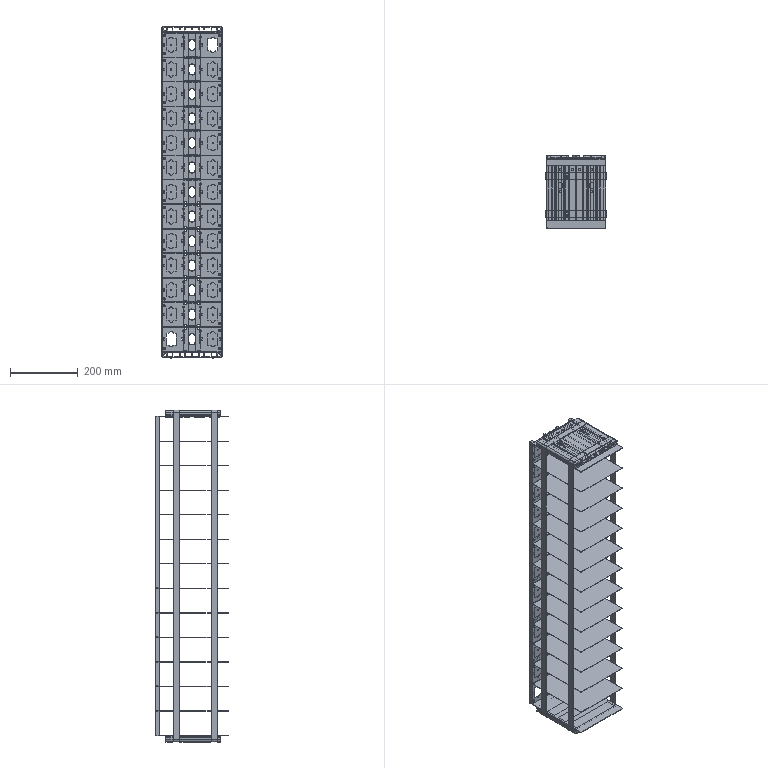Part | NX | features BREP 9 | 38 solids | 5048 faces | volume 1560221 mm3 | plane 2914 | cylinder 2134 | commonest cylinder face diameters 2 x433 4 x388 3 x204 6 x176 0.6 x164 10 x106